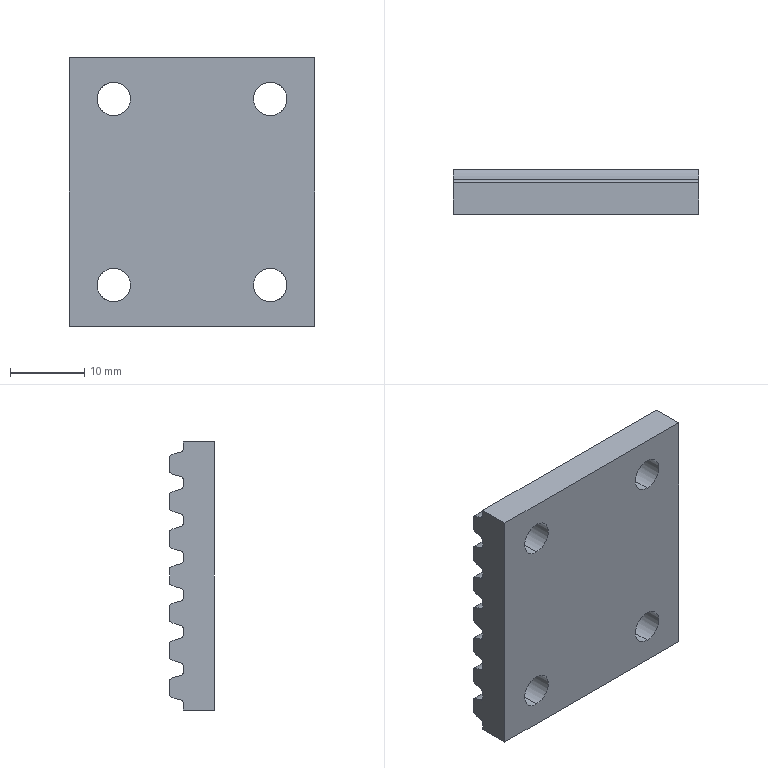Part | SolidWorks | features ICE 2, MoveFace 2, BaseBody 1, HoleWzd 1 | 1 solid | 76 faces | box 33 x 6 x 36 mm | volume 5895 mm3 | cylinder 52 | plane 24 | commonest cylinder face diameters 1 x22 6.522 x22 4.5 x8